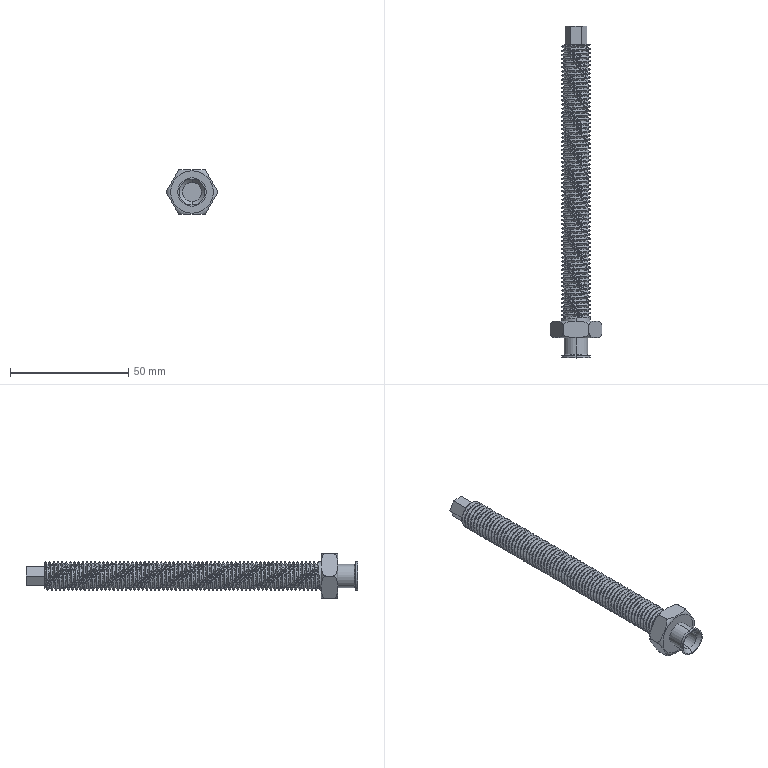Part | NX | features solid 2 | 1 solid | 172 faces | box 21.939 x 140.6 x 19 mm | volume 17803 mm3 | cylinder 141 | plane 20 | torus 4 | cone 4 | spline 3 | commonest cylinder face diameters 12 x137 8 x2 10 x2